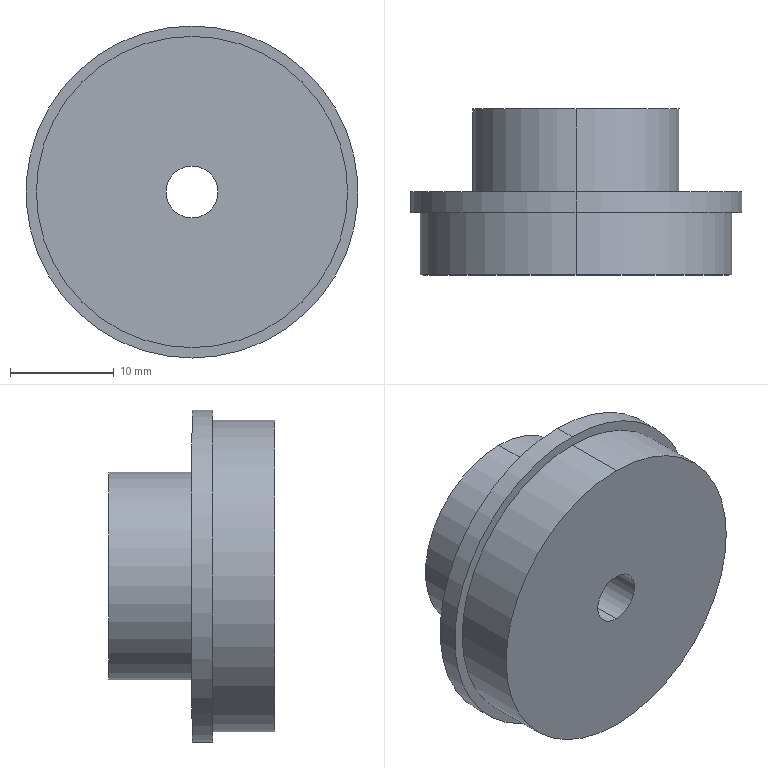Part | STEP file | BCC3 H16_4 | 1 solid | 12 faces | box 32 x 16 x 32 mm | volume 8049 mm3 | cylinder 8 | plane 4 | commonest cylinder face diameters 5 x2 20 x2 30 x2 32 x2
STEP:
#1=CARTESIAN_POINT('',(0.,0.,0.));
#2=DIRECTION('',(0.,0.,1.));
#3=DIRECTION('',(1.,0.,0.));
#4=AXIS2_PLACEMENT_3D('',#1,#2,#3);
#5=CARTESIAN_POINT('',(0.,0.,2.5));
#6=VERTEX_POINT('',#5);
#7=CARTESIAN_POINT('',(0.,16.,2.5));
#8=VERTEX_POINT('',#7);
#9=CARTESIAN_POINT('',(0.,16.,2.5));
#10=DIRECTION('',(0.,1.,0.));
#11=VECTOR('',#10,1.);
#12=LINE('',#9,#11);
#13=CARTESIAN_POINT('',(0.,16.,0.));
#14=DIRECTION('',(0.,1.,0.));
#15=DIRECTION('',(0.,0.,1.));
#16=AXIS2_PLACEMENT_3D('',#13,#14,#15);
#17=CYLINDRICAL_SURFACE('',#16,2.5);
#18=CARTESIAN_POINT('',(6.283,0.));
#19=DIRECTION('',(0.,1.));
#20=VECTOR('',#19,1.);
#21=LINE('',#18,#20);
#22=(GEOMETRIC_REPRESENTATION_CONTEXT(2)PARAMETRIC_REPRESENTATION_CONTEXT()REPRESENTATION_CONTEXT('',''));
#23=DEFINITIONAL_REPRESENTATION('',(#21),#22);
#24=PCURVE('',#17,#23);
#25=CARTESIAN_POINT('',(0.,16.,0.));
#26=DIRECTION('',(0.,1.,0.));
#27=DIRECTION('',(0.,0.,1.));
#28=AXIS2_PLACEMENT_3D('',#25,#26,#27);
#29=CYLINDRICAL_SURFACE('',#28,2.5);
#30=CARTESIAN_POINT('',(0.,0.));
#31=DIRECTION('',(0.,1.));
#32=VECTOR('',#31,1.);
#33=LINE('',#30,#32);
#34=(GEOMETRIC_REPRESENTATION_CONTEXT(2)PARAMETRIC_REPRESENTATION_CONTEXT()REPRESENTATION_CONTEXT('',''));
#35=DEFINITIONAL_REPRESENTATION('',(#33),#34);
#36=PCURVE('',#29,#35);
#37=SURFACE_CURVE('',#12,(#24,#36),.PCURVE_S1.);
#38=EDGE_CURVE('',#6,#8,#37,.T.);
#39=ORIENTED_EDGE('',*,*,#38,.T.);
#40=CARTESIAN_POINT('',(0.,16.,-2.5));
#41=VERTEX_POINT('',#40);
#42=CARTESIAN_POINT('',(0.,16.,0.));
#43=DIRECTION('',(0.,1.,0.));
#44=DIRECTION('',(0.,0.,1.));
#45=AXIS2_PLACEMENT_3D('',#42,#43,#44);
#46=CIRCLE('',#45,2.5);
#47=CARTESIAN_POINT('',(0.,0.));
#48=DIRECTION('',(1.,0.));
#49=VECTOR('',#48,1.);
#50=LINE('',#47,#49);
#51=(GEOMETRIC_REPRESENTATION_CONTEXT(2)PARAMETRIC_REPRESENTATION_CONTEXT()REPRESENTATION_CONTEXT('',''));
#52=DEFINITIONAL_REPRESENTATION('',(#50),#51);
#53=PCURVE('',#17,#52);
#54=CARTESIAN_POINT('',(0.,16.,0.));
#55=DIRECTION('',(0.,1.,0.));
#56=DIRECTION('',(0.,0.,1.));
#57=AXIS2_PLACEMENT_3D('',#54,#55,#56);
#58=PLANE('',#57);
#59=CARTESIAN_POINT('',(0.,0.));
#60=DIRECTION('',(1.,0.));
#61=AXIS2_PLACEMENT_2D('',#59,#60);
#62=CIRCLE('',#61,2.5);
#63=(GEOMETRIC_REPRESENTATION_CONTEXT(2)PARAMETRIC_REPRESENTATION_CONTEXT()REPRESENTATION_CONTEXT('',''));
#64=DEFINITIONAL_REPRESENTATION('',(#62),#63);
#65=PCURVE('',#58,#64);
#66=SURFACE_CURVE('',#46,(#53,#65),.PCURVE_S1.);
#67=EDGE_CURVE('',#41,#8,#66,.T.);
#68=ORIENTED_EDGE('',*,*,#67,.F.);
#69=CARTESIAN_POINT('',(0.,0.,-2.5));
#70=VERTEX_POINT('',#69);
#71=CARTESIAN_POINT('',(0.,16.,-2.5));
#72=DIRECTION('',(0.,1.,0.));
#73=VECTOR('',#72,1.);
#74=LINE('',#71,#73);
#75=CARTESIAN_POINT('',(3.142,0.));
#76=DIRECTION('',(0.,1.));
#77=VECTOR('',#76,1.);
#78=LINE('',#75,#77);
#79=(GEOMETRIC_REPRESENTATION_CONTEXT(2)PARAMETRIC_REPRESENTATION_CONTEXT()REPRESENTATION_CONTEXT('',''));
#80=DEFINITIONAL_REPRESENTATION('',(#78),#79);
#81=PCURVE('',#17,#80);
#82=CARTESIAN_POINT('',(3.142,0.));
#83=DIRECTION('',(0.,1.));
#84=VECTOR('',#83,1.);
#85=LINE('',#82,#84);
#86=(GEOMETRIC_REPRESENTATION_CONTEXT(2)PARAMETRIC_REPRESENTATION_CONTEXT()REPRESENTATION_CONTEXT('',''));
#87=DEFINITIONAL_REPRESENTATION('',(#85),#86);
#88=PCURVE('',#29,#87);
#89=SURFACE_CURVE('',#74,(#81,#88),.PCURVE_S1.);
#90=EDGE_CURVE('',#70,#41,#89,.T.);
#91=ORIENTED_EDGE('',*,*,#90,.F.);
#92=CARTESIAN_POINT('',(0.,0.,0.));
#93=DIRECTION('',(0.,1.,0.));
#94=DIRECTION('',(0.,0.,1.));
#95=AXIS2_PLACEMENT_3D('',#92,#93,#94);
#96=CIRCLE('',#95,2.5);
#97=CARTESIAN_POINT('',(0.,-16.));
#98=DIRECTION('',(1.,0.));
#99=VECTOR('',#98,1.);
#100=LINE('',#97,#99);
#101=(GEOMETRIC_REPRESENTATION_CONTEXT(2)PARAMETRIC_REPRESENTATION_CONTEXT()REPRESENTATION_CONTEXT('',''));
#102=DEFINITIONAL_REPRESENTATION('',(#100),#101);
#103=PCURVE('',#17,#102);
#104=CARTESIAN_POINT('',(0.,0.,0.));
#105=DIRECTION('',(0.,1.,0.));
#106=DIRECTION('',(0.,0.,1.));
#107=AXIS2_PLACEMENT_3D('',#104,#105,#106);
#108=PLANE('',#107);
#109=CARTESIAN_POINT('',(0.,0.));
#110=DIRECTION('',(1.,0.));
#111=AXIS2_PLACEMENT_2D('',#109,#110);
#112=CIRCLE('',#111,2.5);
#113=(GEOMETRIC_REPRESENTATION_CONTEXT(2)PARAMETRIC_REPRESENTATION_CONTEXT()REPRESENTATION_CONTEXT('',''));
#114=DEFINITIONAL_REPRESENTATION('',(#112),#113);
#115=PCURVE('',#108,#114);
#116=SURFACE_CURVE('',#96,(#103,#115),.PCURVE_S1.);
#117=EDGE_CURVE('',#70,#6,#116,.T.);
#118=ORIENTED_EDGE('',*,*,#117,.T.);
#119=EDGE_LOOP('',(#39,#68,#91,#118));
#120=FACE_BOUND('',#119,.F.);
#121=ADVANCED_FACE('',(#120),#17,.F.);
#122=CARTESIAN_POINT('',(0.,16.,10.));
#123=VERTEX_POINT('',#122);
#124=CARTESIAN_POINT('',(0.,16.,-10.));
#125=VERTEX_POINT('',#124);
#126=CARTESIAN_POINT('',(0.,16.,0.));
#127=DIRECTION('',(0.,1.,0.));
#128=DIRECTION('',(0.,0.,1.));
#129=AXIS2_PLACEMENT_3D('',#126,#127,#128);
#130=CIRCLE('',#129,10.);
#131=CARTESIAN_POINT('',(0.,16.,0.));
#132=DIRECTION('',(0.,-1.,0.));
#133=DIRECTION('',(0.,0.,-1.));
#134=AXIS2_PLACEMENT_3D('',#131,#132,#133);
#135=CYLINDRICAL_SURFACE('',#134,10.);
#136=CARTESIAN_POINT('',(3.142,0.));
#137=DIRECTION('',(-1.,0.));
#138=VECTOR('',#137,1.);
#139=LINE('',#136,#138);
#140=(GEOMETRIC_REPRESENTATION_CONTEXT(2)PARAMETRIC_REPRESENTATION_CONTEXT()REPRESENTATION_CONTEXT('',''));
#141=DEFINITIONAL_REPRESENTATION('',(#139),#140);
#142=PCURVE('',#135,#141);
#143=CARTESIAN_POINT('',(0.,0.));
#144=DIRECTION('',(1.,0.));
#145=AXIS2_PLACEMENT_2D('',#143,#144);
#146=CIRCLE('',#145,10.);
#147=(GEOMETRIC_REPRESENTATION_CONTEXT(2)PARAMETRIC_REPRESENTATION_CONTEXT()REPRESENTATION_CONTEXT('',''));
#148=DEFINITIONAL_REPRESENTATION('',(#146),#147);
#149=PCURVE('',#58,#148);
#150=SURFACE_CURVE('',#130,(#142,#149),.PCURVE_S1.);
#151=EDGE_CURVE('',#123,#125,#150,.T.);
#152=ORIENTED_EDGE('',*,*,#151,.F.);
#153=CARTESIAN_POINT('',(0.,8.,10.));
#154=VERTEX_POINT('',#153);
#155=CARTESIAN_POINT('',(0.,16.,10.));
#156=DIRECTION('',(0.,-1.,0.));
#157=VECTOR('',#156,1.);
#158=LINE('',#155,#157);
#159=CARTESIAN_POINT('',(3.142,0.));
#160=DIRECTION('',(0.,1.));
#161=VECTOR('',#160,1.);
#162=LINE('',#159,#161);
#163=(GEOMETRIC_REPRESENTATION_CONTEXT(2)PARAMETRIC_REPRESENTATION_CONTEXT()REPRESENTATION_CONTEXT('',''));
#164=DEFINITIONAL_REPRESENTATION('',(#162),#163);
#165=PCURVE('',#135,#164);
#166=CARTESIAN_POINT('',(0.,16.,0.));
#167=DIRECTION('',(0.,-1.,0.));
#168=DIRECTION('',(0.,0.,-1.));
#169=AXIS2_PLACEMENT_3D('',#166,#167,#168);
#170=CYLINDRICAL_SURFACE('',#169,10.);
#171=CARTESIAN_POINT('',(3.142,0.));
#172=DIRECTION('',(0.,1.));
#173=VECTOR('',#172,1.);
#174=LINE('',#171,#173);
#175=(GEOMETRIC_REPRESENTATION_CONTEXT(2)PARAMETRIC_REPRESENTATION_CONTEXT()REPRESENTATION_CONTEXT('',''));
#176=DEFINITIONAL_REPRESENTATION('',(#174),#175);
#177=PCURVE('',#170,#176);
#178=SURFACE_CURVE('',#158,(#165,#177),.PCURVE_S1.);
#179=EDGE_CURVE('',#123,#154,#178,.T.);
#180=ORIENTED_EDGE('',*,*,#179,.T.);
#181=CARTESIAN_POINT('',(0.,8.,-10.));
#182=VERTEX_POINT('',#181);
#183=CARTESIAN_POINT('',(0.,8.,0.));
#184=DIRECTION('',(0.,1.,0.));
#185=DIRECTION('',(0.,0.,1.));
#186=AXIS2_PLACEMENT_3D('',#183,#184,#185);
#187=CIRCLE('',#186,10.);
#188=CARTESIAN_POINT('',(3.142,8.));
#189=DIRECTION('',(-1.,0.));
#190=VECTOR('',#189,1.);
#191=LINE('',#188,#190);
#192=(GEOMETRIC_REPRESENTATION_CONTEXT(2)PARAMETRIC_REPRESENTATION_CONTEXT()REPRESENTATION_CONTEXT('',''));
#193=DEFINITIONAL_REPRESENTATION('',(#191),#192);
#194=PCURVE('',#135,#193);
#195=CARTESIAN_POINT('',(0.,8.,0.));
#196=DIRECTION('',(0.,1.,0.));
#197=DIRECTION('',(0.,0.,1.));
#198=AXIS2_PLACEMENT_3D('',#195,#196,#197);
#199=PLANE('',#198);
#200=CARTESIAN_POINT('',(0.,0.));
#201=DIRECTION('',(1.,0.));
#202=AXIS2_PLACEMENT_2D('',#200,#201);
#203=CIRCLE('',#202,10.);
#204=(GEOMETRIC_REPRESENTATION_CONTEXT(2)PARAMETRIC_REPRESENTATION_CONTEXT()REPRESENTATION_CONTEXT('',''));
#205=DEFINITIONAL_REPRESENTATION('',(#203),#204);
#206=PCURVE('',#199,#205);
#207=SURFACE_CURVE('',#187,(#194,#206),.PCURVE_S1.);
#208=EDGE_CURVE('',#154,#182,#207,.T.);
#209=ORIENTED_EDGE('',*,*,#208,.T.);
#210=CARTESIAN_POINT('',(0.,16.,-10.));
#211=DIRECTION('',(0.,-1.,0.));
#212=VECTOR('',#211,1.);
#213=LINE('',#210,#212);
#214=CARTESIAN_POINT('',(0.,0.));
#215=DIRECTION('',(0.,1.));
#216=VECTOR('',#215,1.);
#217=LINE('',#214,#216);
#218=(GEOMETRIC_REPRESENTATION_CONTEXT(2)PARAMETRIC_REPRESENTATION_CONTEXT()REPRESENTATION_CONTEXT('',''));
#219=DEFINITIONAL_REPRESENTATION('',(#217),#218);
#220=PCURVE('',#135,#219);
#221=CARTESIAN_POINT('',(6.283,0.));
#222=DIRECTION('',(0.,1.));
#223=VECTOR('',#222,1.);
#224=LINE('',#221,#223);
#225=(GEOMETRIC_REPRESENTATION_CONTEXT(2)PARAMETRIC_REPRESENTATION_CONTEXT()REPRESENTATION_CONTEXT('',''));
#226=DEFINITIONAL_REPRESENTATION('',(#224),#225);
#227=PCURVE('',#170,#226);
#228=SURFACE_CURVE('',#213,(#220,#227),.PCURVE_S1.);
#229=EDGE_CURVE('',#125,#182,#228,.T.);
#230=ORIENTED_EDGE('',*,*,#229,.F.);
#231=EDGE_LOOP('',(#152,#180,#209,#230));
#232=FACE_BOUND('',#231,.T.);
#233=ADVANCED_FACE('',(#232),#135,.T.);
#234=CARTESIAN_POINT('',(0.,8.,16.));
#235=VERTEX_POINT('',#234);
#236=CARTESIAN_POINT('',(0.,8.,-16.));
#237=VERTEX_POINT('',#236);
#238=CARTESIAN_POINT('',(0.,8.,0.));
#239=DIRECTION('',(0.,1.,0.));
#240=DIRECTION('',(0.,0.,1.));
#241=AXIS2_PLACEMENT_3D('',#238,#239,#240);
#242=CIRCLE('',#241,16.);
#243=CARTESIAN_POINT('',(0.,8.,0.));
#244=DIRECTION('',(0.,-1.,0.));
#245=DIRECTION('',(0.,0.,-1.));
#246=AXIS2_PLACEMENT_3D('',#243,#244,#245);
#247=CYLINDRICAL_SURFACE('',#246,16.);
#248=CARTESIAN_POINT('',(3.142,0.));
#249=DIRECTION('',(-1.,0.));
#250=VECTOR('',#249,1.);
#251=LINE('',#248,#250);
#252=(GEOMETRIC_REPRESENTATION_CONTEXT(2)PARAMETRIC_REPRESENTATION_CONTEXT()REPRESENTATION_CONTEXT('',''));
#253=DEFINITIONAL_REPRESENTATION('',(#251),#252);
#254=PCURVE('',#247,#253);
#255=CARTESIAN_POINT('',(0.,0.));
#256=DIRECTION('',(1.,0.));
#257=AXIS2_PLACEMENT_2D('',#255,#256);
#258=CIRCLE('',#257,16.);
#259=(GEOMETRIC_REPRESENTATION_CONTEXT(2)PARAMETRIC_REPRESENTATION_CONTEXT()REPRESENTATION_CONTEXT('',''));
#260=DEFINITIONAL_REPRESENTATION('',(#258),#259);
#261=PCURVE('',#199,#260);
#262=SURFACE_CURVE('',#242,(#254,#261),.PCURVE_S1.);
#263=EDGE_CURVE('',#235,#237,#262,.T.);
#264=ORIENTED_EDGE('',*,*,#263,.F.);
#265=CARTESIAN_POINT('',(0.,6.,16.));
#266=VERTEX_POINT('',#265);
#267=CARTESIAN_POINT('',(0.,8.,16.));
#268=DIRECTION('',(0.,-1.,0.));
#269=VECTOR('',#268,1.);
#270=LINE('',#267,#269);
#271=CARTESIAN_POINT('',(3.142,0.));
#272=DIRECTION('',(0.,1.));
#273=VECTOR('',#272,1.);
#274=LINE('',#271,#273);
#275=(GEOMETRIC_REPRESENTATION_CONTEXT(2)PARAMETRIC_REPRESENTATION_CONTEXT()REPRESENTATION_CONTEXT('',''));
#276=DEFINITIONAL_REPRESENTATION('',(#274),#275);
#277=PCURVE('',#247,#276);
#278=CARTESIAN_POINT('',(0.,8.,0.));
#279=DIRECTION('',(0.,-1.,0.));
#280=DIRECTION('',(0.,0.,-1.));
#281=AXIS2_PLACEMENT_3D('',#278,#279,#280);
#282=CYLINDRICAL_SURFACE('',#281,16.);
#283=CARTESIAN_POINT('',(3.142,0.));
#284=DIRECTION('',(0.,1.));
#285=VECTOR('',#284,1.);
#286=LINE('',#283,#285);
#287=(GEOMETRIC_REPRESENTATION_CONTEXT(2)PARAMETRIC_REPRESENTATION_CONTEXT()REPRESENTATION_CONTEXT('',''));
#288=DEFINITIONAL_REPRESENTATION('',(#286),#287);
#289=PCURVE('',#282,#288);
#290=SURFACE_CURVE('',#270,(#277,#289),.PCURVE_S1.);
#291=EDGE_CURVE('',#235,#266,#290,.T.);
#292=ORIENTED_EDGE('',*,*,#291,.T.);
#293=CARTESIAN_POINT('',(0.,6.,-16.));
#294=VERTEX_POINT('',#293);
#295=CARTESIAN_POINT('',(0.,6.,0.));
#296=DIRECTION('',(0.,1.,0.));
#297=DIRECTION('',(0.,0.,1.));
#298=AXIS2_PLACEMENT_3D('',#295,#296,#297);
#299=CIRCLE('',#298,16.);
#300=CARTESIAN_POINT('',(3.142,2.));
#301=DIRECTION('',(-1.,0.));
#302=VECTOR('',#301,1.);
#303=LINE('',#300,#302);
#304=(GEOMETRIC_REPRESENTATION_CONTEXT(2)PARAMETRIC_REPRESENTATION_CONTEXT()REPRESENTATION_CONTEXT('',''));
#305=DEFINITIONAL_REPRESENTATION('',(#303),#304);
#306=PCURVE('',#247,#305);
#307=CARTESIAN_POINT('',(0.,6.,0.));
#308=DIRECTION('',(0.,1.,0.));
#309=DIRECTION('',(0.,0.,1.));
#310=AXIS2_PLACEMENT_3D('',#307,#308,#309);
#311=PLANE('',#310);
#312=CARTESIAN_POINT('',(0.,0.));
#313=DIRECTION('',(1.,0.));
#314=AXIS2_PLACEMENT_2D('',#312,#313);
#315=CIRCLE('',#314,16.);
#316=(GEOMETRIC_REPRESENTATION_CONTEXT(2)PARAMETRIC_REPRESENTATION_CONTEXT()REPRESENTATION_CONTEXT('',''));
#317=DEFINITIONAL_REPRESENTATION('',(#315),#316);
#318=PCURVE('',#311,#317);
#319=SURFACE_CURVE('',#299,(#306,#318),.PCURVE_S1.);
#320=EDGE_CURVE('',#266,#294,#319,.T.);
#321=ORIENTED_EDGE('',*,*,#320,.T.);
#322=CARTESIAN_POINT('',(0.,8.,-16.));
#323=DIRECTION('',(0.,-1.,0.));
#324=VECTOR('',#323,1.);
#325=LINE('',#322,#324);
#326=CARTESIAN_POINT('',(0.,0.));
#327=DIRECTION('',(0.,1.));
#328=VECTOR('',#327,1.);
#329=LINE('',#326,#328);
#330=(GEOMETRIC_REPRESENTATION_CONTEXT(2)PARAMETRIC_REPRESENTATION_CONTEXT()REPRESENTATION_CONTEXT('',''));
#331=DEFINITIONAL_REPRESENTATION('',(#329),#330);
#332=PCURVE('',#247,#331);
#333=CARTESIAN_POINT('',(6.283,0.));
#334=DIRECTION('',(0.,1.));
#335=VECTOR('',#334,1.);
#336=LINE('',#333,#335);
#337=(GEOMETRIC_REPRESENTATION_CONTEXT(2)PARAMETRIC_REPRESENTATION_CONTEXT()REPRESENTATION_CONTEXT('',''));
#338=DEFINITIONAL_REPRESENTATION('',(#336),#337);
#339=PCURVE('',#282,#338);
#340=SURFACE_CURVE('',#325,(#332,#339),.PCURVE_S1.);
#341=EDGE_CURVE('',#237,#294,#340,.T.);
#342=ORIENTED_EDGE('',*,*,#341,.F.);
#343=EDGE_LOOP('',(#264,#292,#321,#342));
#344=FACE_BOUND('',#343,.T.);
#345=ADVANCED_FACE('',(#344),#247,.T.);
#346=CARTESIAN_POINT('',(0.,6.,15.));
#347=VERTEX_POINT('',#346);
#348=CARTESIAN_POINT('',(0.,6.,-15.));
#349=VERTEX_POINT('',#348);
#350=CARTESIAN_POINT('',(0.,6.,0.));
#351=DIRECTION('',(0.,1.,0.));
#352=DIRECTION('',(0.,0.,1.));
#353=AXIS2_PLACEMENT_3D('',#350,#351,#352);
#354=CIRCLE('',#353,15.);
#355=CARTESIAN_POINT('',(0.,6.,0.));
#356=DIRECTION('',(0.,-1.,0.));
#357=DIRECTION('',(0.,0.,-1.));
#358=AXIS2_PLACEMENT_3D('',#355,#356,#357);
#359=CYLINDRICAL_SURFACE('',#358,15.);
#360=CARTESIAN_POINT('',(3.142,0.));
#361=DIRECTION('',(-1.,0.));
#362=VECTOR('',#361,1.);
#363=LINE('',#360,#362);
#364=(GEOMETRIC_REPRESENTATION_CONTEXT(2)PARAMETRIC_REPRESENTATION_CONTEXT()REPRESENTATION_CONTEXT('',''));
#365=DEFINITIONAL_REPRESENTATION('',(#363),#364);
#366=PCURVE('',#359,#365);
#367=CARTESIAN_POINT('',(0.,0.));
#368=DIRECTION('',(1.,0.));
#369=AXIS2_PLACEMENT_2D('',#367,#368);
#370=CIRCLE('',#369,15.);
#371=(GEOMETRIC_REPRESENTATION_CONTEXT(2)PARAMETRIC_REPRESENTATION_CONTEXT()REPRESENTATION_CONTEXT('',''));
#372=DEFINITIONAL_REPRESENTATION('',(#370),#371);
#373=PCURVE('',#311,#372);
#374=SURFACE_CURVE('',#354,(#366,#373),.PCURVE_S1.);
#375=EDGE_CURVE('',#347,#349,#374,.T.);
#376=ORIENTED_EDGE('',*,*,#375,.F.);
#377=CARTESIAN_POINT('',(0.,0.,15.));
#378=VERTEX_POINT('',#377);
#379=CARTESIAN_POINT('',(0.,6.,15.));
#380=DIRECTION('',(0.,-1.,0.));
#381=VECTOR('',#380,1.);
#382=LINE('',#379,#381);
#383=CARTESIAN_POINT('',(3.142,0.));
#384=DIRECTION('',(0.,1.));
#385=VECTOR('',#384,1.);
#386=LINE('',#383,#385);
#387=(GEOMETRIC_REPRESENTATION_CONTEXT(2)PARAMETRIC_REPRESENTATION_CONTEXT()REPRESENTATION_CONTEXT('',''));
#388=DEFINITIONAL_REPRESENTATION('',(#386),#387);
#389=PCURVE('',#359,#388);
#390=CARTESIAN_POINT('',(0.,6.,0.));
#391=DIRECTION('',(0.,-1.,0.));
#392=DIRECTION('',(0.,0.,-1.));
#393=AXIS2_PLACEMENT_3D('',#390,#391,#392);
#394=CYLINDRICAL_SURFACE('',#393,15.);
#395=CARTESIAN_POINT('',(3.142,0.));
#396=DIRECTION('',(0.,1.));
#397=VECTOR('',#396,1.);
#398=LINE('',#395,#397);
#399=(GEOMETRIC_REPRESENTATION_CONTEXT(2)PARAMETRIC_REPRESENTATION_CONTEXT()REPRESENTATION_CONTEXT('',''));
#400=DEFINITIONAL_REPRESENTATION('',(#398),#399);
#401=PCURVE('',#394,#400);
#402=SURFACE_CURVE('',#382,(#389,#401),.PCURVE_S1.);
#403=EDGE_CURVE('',#347,#378,#402,.T.);
#404=ORIENTED_EDGE('',*,*,#403,.T.);
#405=CARTESIAN_POINT('',(0.,0.,-15.));
#406=VERTEX_POINT('',#405);
#407=CARTESIAN_POINT('',(0.,0.,0.));
#408=DIRECTION('',(0.,1.,0.));
#409=DIRECTION('',(0.,0.,1.));
#410=AXIS2_PLACEMENT_3D('',#407,#408,#409);
#411=CIRCLE('',#410,15.);
#412=CARTESIAN_POINT('',(3.142,6.));
#413=DIRECTION('',(-1.,0.));
#414=VECTOR('',#413,1.);
#415=LINE('',#412,#414);
#416=(GEOMETRIC_REPRESENTATION_CONTEXT(2)PARAMETRIC_REPRESENTATION_CONTEXT()REPRESENTATION_CONTEXT('',''));
#417=DEFINITIONAL_REPRESENTATION('',(#415),#416);
#418=PCURVE('',#359,#417);
#419=CARTESIAN_POINT('',(0.,0.));
#420=DIRECTION('',(1.,0.));
#421=AXIS2_PLACEMENT_2D('',#419,#420);
#422=CIRCLE('',#421,15.);
#423=(GEOMETRIC_REPRESENTATION_CONTEXT(2)PARAMETRIC_REPRESENTATION_CONTEXT()REPRESENTATION_CONTEXT('',''));
#424=DEFINITIONAL_REPRESENTATION('',(#422),#423);
#425=PCURVE('',#108,#424);
#426=SURFACE_CURVE('',#411,(#418,#425),.PCURVE_S1.);
#427=EDGE_CURVE('',#378,#406,#426,.T.);
#428=ORIENTED_EDGE('',*,*,#427,.T.);
#429=CARTESIAN_POINT('',(0.,6.,-15.));
#430=DIRECTION('',(0.,-1.,0.));
#431=VECTOR('',#430,1.);
#432=LINE('',#429,#431);
#433=CARTESIAN_POINT('',(0.,0.));
#434=DIRECTION('',(0.,1.));
#435=VECTOR('',#434,1.);
#436=LINE('',#433,#435);
#437=(GEOMETRIC_REPRESENTATION_CONTEXT(2)PARAMETRIC_REPRESENTATION_CONTEXT()REPRESENTATION_CONTEXT('',''));
#438=DEFINITIONAL_REPRESENTATION('',(#436),#437);
#439=PCURVE('',#359,#438);
#440=CARTESIAN_POINT('',(6.283,0.));
#441=DIRECTION('',(0.,1.));
#442=VECTOR('',#441,1.);
#443=LINE('',#440,#442);
#444=(GEOMETRIC_REPRESENTATION_CONTEXT(2)PARAMETRIC_REPRESENTATION_CONTEXT()REPRESENTATION_CONTEXT('',''));
#445=DEFINITIONAL_REPRESENTATION('',(#443),#444);
#446=PCURVE('',#394,#445);
#447=SURFACE_CURVE('',#432,(#439,#446),.PCURVE_S1.);
#448=EDGE_CURVE('',#349,#406,#447,.T.);
#449=ORIENTED_EDGE('',*,*,#448,.F.);
#450=EDGE_LOOP('',(#376,#404,#428,#449));
#451=FACE_BOUND('',#450,.T.);
#452=ADVANCED_FACE('',(#451),#359,.T.);
#453=CARTESIAN_POINT('',(0.,8.,0.));
#454=DIRECTION('',(0.,1.,0.));
#455=DIRECTION('',(0.,0.,1.));
#456=AXIS2_PLACEMENT_3D('',#453,#454,#455);
#457=CIRCLE('',#456,16.);
#458=CARTESIAN_POINT('',(0.,0.));
#459=DIRECTION('',(1.,0.));
#460=AXIS2_PLACEMENT_2D('',#458,#459);
#461=CIRCLE('',#460,16.);
#462=(GEOMETRIC_REPRESENTATION_CONTEXT(2)PARAMETRIC_REPRESENTATION_CONTEXT()REPRESENTATION_CONTEXT('',''));
#463=DEFINITIONAL_REPRESENTATION('',(#461),#462);
#464=PCURVE('',#199,#463);
#465=CARTESIAN_POINT('',(9.425,0.));
#466=DIRECTION('',(-1.,0.));
#467=VECTOR('',#466,1.);
#468=LINE('',#465,#467);
#469=(GEOMETRIC_REPRESENTATION_CONTEXT(2)PARAMETRIC_REPRESENTATION_CONTEXT()REPRESENTATION_CONTEXT('',''));
#470=DEFINITIONAL_REPRESENTATION('',(#468),#469);
#471=PCURVE('',#282,#470);
#472=SURFACE_CURVE('',#457,(#464,#471),.PCURVE_S1.);
#473=EDGE_CURVE('',#237,#235,#472,.T.);
#474=ORIENTED_EDGE('',*,*,#473,.T.);
#475=ORIENTED_EDGE('',*,*,#263,.T.);
#476=EDGE_LOOP('',(#474,#475));
#477=FACE_BOUND('',#476,.T.);
#478=CARTESIAN_POINT('',(0.,8.,0.));
#479=DIRECTION('',(0.,1.,0.));
#480=DIRECTION('',(0.,0.,1.));
#481=AXIS2_PLACEMENT_3D('',#478,#479,#480);
#482=CIRCLE('',#481,10.);
#483=CARTESIAN_POINT('',(0.,0.));
#484=DIRECTION('',(1.,0.));
#485=AXIS2_PLACEMENT_2D('',#483,#484);
#486=CIRCLE('',#485,10.);
#487=(GEOMETRIC_REPRESENTATION_CONTEXT(2)PARAMETRIC_REPRESENTATION_CONTEXT()REPRESENTATION_CONTEXT('',''));
#488=DEFINITIONAL_REPRESENTATION('',(#486),#487);
#489=PCURVE('',#199,#488);
#490=CARTESIAN_POINT('',(9.425,8.));
#491=DIRECTION('',(-1.,0.));
#492=VECTOR('',#491,1.);
#493=LINE('',#490,#492);
#494=(GEOMETRIC_REPRESENTATION_CONTEXT(2)PARAMETRIC_REPRESENTATION_CONTEXT()REPRESENTATION_CONTEXT('',''));
#495=DEFINITIONAL_REPRESENTATION('',(#493),#494);
#496=PCURVE('',#170,#495);
#497=SURFACE_CURVE('',#482,(#489,#496),.PCURVE_S1.);
#498=EDGE_CURVE('',#182,#154,#497,.T.);
#499=ORIENTED_EDGE('',*,*,#498,.F.);
#500=ORIENTED_EDGE('',*,*,#208,.F.);
#501=EDGE_LOOP('',(#499,#500));
#502=FACE_BOUND('',#501,.T.);
#503=ADVANCED_FACE('',(#477,#502),#199,.T.);
#504=ORIENTED_EDGE('',*,*,#403,.F.);
#505=CARTESIAN_POINT('',(0.,6.,0.));
#506=DIRECTION('',(0.,1.,0.));
#507=DIRECTION('',(0.,0.,1.));
#508=AXIS2_PLACEMENT_3D('',#505,#506,#507);
#509=CIRCLE('',#508,15.);
#510=CARTESIAN_POINT('',(9.425,0.));
#511=DIRECTION('',(-1.,0.));
#512=VECTOR('',#511,1.);
#513=LINE('',#510,#512);
#514=(GEOMETRIC_REPRESENTATION_CONTEXT(2)PARAMETRIC_REPRESENTATION_CONTEXT()REPRESENTATION_CONTEXT('',''));
#515=DEFINITIONAL_REPRESENTATION('',(#513),#514);
#516=PCURVE('',#394,#515);
#517=CARTESIAN_POINT('',(0.,0.));
#518=DIRECTION('',(1.,0.));
#519=AXIS2_PLACEMENT_2D('',#517,#518);
#520=CIRCLE('',#519,15.);
#521=(GEOMETRIC_REPRESENTATION_CONTEXT(2)PARAMETRIC_REPRESENTATION_CONTEXT()REPRESENTATION_CONTEXT('',''));
#522=DEFINITIONAL_REPRESENTATION('',(#520),#521);
#523=PCURVE('',#311,#522);
#524=SURFACE_CURVE('',#509,(#516,#523),.PCURVE_S1.);
#525=EDGE_CURVE('',#349,#347,#524,.T.);
#526=ORIENTED_EDGE('',*,*,#525,.F.);
#527=ORIENTED_EDGE('',*,*,#448,.T.);
#528=CARTESIAN_POINT('',(0.,0.,0.));
#529=DIRECTION('',(0.,1.,0.));
#530=DIRECTION('',(0.,0.,1.));
#531=AXIS2_PLACEMENT_3D('',#528,#529,#530);
#532=CIRCLE('',#531,15.);
#533=CARTESIAN_POINT('',(9.425,6.));
#534=DIRECTION('',(-1.,0.));
#535=VECTOR('',#534,1.);
#536=LINE('',#533,#535);
#537=(GEOMETRIC_REPRESENTATION_CONTEXT(2)PARAMETRIC_REPRESENTATION_CONTEXT()REPRESENTATION_CONTEXT('',''));
#538=DEFINITIONAL_REPRESENTATION('',(#536),#537);
#539=PCURVE('',#394,#538);
#540=CARTESIAN_POINT('',(0.,0.));
#541=DIRECTION('',(1.,0.));
#542=AXIS2_PLACEMENT_2D('',#540,#541);
#543=CIRCLE('',#542,15.);
#544=(GEOMETRIC_REPRESENTATION_CONTEXT(2)PARAMETRIC_REPRESENTATION_CONTEXT()REPRESENTATION_CONTEXT('',''));
#545=DEFINITIONAL_REPRESENTATION('',(#543),#544);
#546=PCURVE('',#108,#545);
#547=SURFACE_CURVE('',#532,(#539,#546),.PCURVE_S1.);
#548=EDGE_CURVE('',#406,#378,#547,.T.);
#549=ORIENTED_EDGE('',*,*,#548,.T.);
#550=EDGE_LOOP('',(#504,#526,#527,#549));
#551=FACE_BOUND('',#550,.T.);
#552=ADVANCED_FACE('',(#551),#394,.T.);
#553=CARTESIAN_POINT('',(0.,0.,0.));
#554=DIRECTION('',(0.,1.,0.));
#555=DIRECTION('',(0.,0.,1.));
#556=AXIS2_PLACEMENT_3D('',#553,#554,#555);
#557=CIRCLE('',#556,2.5);
#558=CARTESIAN_POINT('',(0.,0.));
#559=DIRECTION('',(1.,0.));
#560=AXIS2_PLACEMENT_2D('',#558,#559);
#561=CIRCLE('',#560,2.5);
#562=(GEOMETRIC_REPRESENTATION_CONTEXT(2)PARAMETRIC_REPRESENTATION_CONTEXT()REPRESENTATION_CONTEXT('',''));
#563=DEFINITIONAL_REPRESENTATION('',(#561),#562);
#564=PCURVE('',#108,#563);
#565=CARTESIAN_POINT('',(0.,-16.));
#566=DIRECTION('',(1.,0.));
#567=VECTOR('',#566,1.);
#568=LINE('',#565,#567);
#569=(GEOMETRIC_REPRESENTATION_CONTEXT(2)PARAMETRIC_REPRESENTATION_CONTEXT()REPRESENTATION_CONTEXT('',''));
#570=DEFINITIONAL_REPRESENTATION('',(#568),#569);
#571=PCURVE('',#29,#570);
#572=SURFACE_CURVE('',#557,(#564,#571),.PCURVE_S1.);
#573=EDGE_CURVE('',#6,#70,#572,.T.);
#574=ORIENTED_EDGE('',*,*,#573,.T.);
#575=ORIENTED_EDGE('',*,*,#117,.T.);
#576=EDGE_LOOP('',(#574,#575));
#577=FACE_BOUND('',#576,.T.);
#578=ORIENTED_EDGE('',*,*,#548,.F.);
#579=ORIENTED_EDGE('',*,*,#427,.F.);
#580=EDGE_LOOP('',(#578,#579));
#581=FACE_BOUND('',#580,.T.);
#582=ADVANCED_FACE('',(#577,#581),#108,.F.);
#583=CARTESIAN_POINT('',(0.,6.,0.));
#584=DIRECTION('',(0.,1.,0.));
#585=DIRECTION('',(0.,0.,1.));
#586=AXIS2_PLACEMENT_3D('',#583,#584,#585);
#587=CIRCLE('',#586,16.);
#588=CARTESIAN_POINT('',(0.,0.));
#589=DIRECTION('',(1.,0.));
#590=AXIS2_PLACEMENT_2D('',#588,#589);
#591=CIRCLE('',#590,16.);
#592=(GEOMETRIC_REPRESENTATION_CONTEXT(2)PARAMETRIC_REPRESENTATION_CONTEXT()REPRESENTATION_CONTEXT('',''));
#593=DEFINITIONAL_REPRESENTATION('',(#591),#592);
#594=PCURVE('',#311,#593);
#595=CARTESIAN_POINT('',(9.425,2.));
#596=DIRECTION('',(-1.,0.));
#597=VECTOR('',#596,1.);
#598=LINE('',#595,#597);
#599=(GEOMETRIC_REPRESENTATION_CONTEXT(2)PARAMETRIC_REPRESENTATION_CONTEXT()REPRESENTATION_CONTEXT('',''));
#600=DEFINITIONAL_REPRESENTATION('',(#598),#599);
#601=PCURVE('',#282,#600);
#602=SURFACE_CURVE('',#587,(#594,#601),.PCURVE_S1.);
#603=EDGE_CURVE('',#294,#266,#602,.T.);
#604=ORIENTED_EDGE('',*,*,#603,.F.);
#605=ORIENTED_EDGE('',*,*,#320,.F.);
#606=EDGE_LOOP('',(#604,#605));
#607=FACE_BOUND('',#606,.T.);
#608=ORIENTED_EDGE('',*,*,#525,.T.);
#609=ORIENTED_EDGE('',*,*,#375,.T.);
#610=EDGE_LOOP('',(#608,#609));
#611=FACE_BOUND('',#610,.T.);
#612=ADVANCED_FACE('',(#607,#611),#311,.F.);
#613=ORIENTED_EDGE('',*,*,#291,.F.);
#614=ORIENTED_EDGE('',*,*,#473,.F.);
#615=ORIENTED_EDGE('',*,*,#341,.T.);
#616=ORIENTED_EDGE('',*,*,#603,.T.);
#617=EDGE_LOOP('',(#613,#614,#615,#616));
#618=FACE_BOUND('',#617,.T.);
#619=ADVANCED_FACE('',(#618),#282,.T.);
#620=ORIENTED_EDGE('',*,*,#179,.F.);
#621=CARTESIAN_POINT('',(0.,16.,0.));
#622=DIRECTION('',(0.,1.,0.));
#623=DIRECTION('',(0.,0.,1.));
#624=AXIS2_PLACEMENT_3D('',#621,#622,#623);
#625=CIRCLE('',#624,10.);
#626=CARTESIAN_POINT('',(9.425,0.));
#627=DIRECTION('',(-1.,0.));
#628=VECTOR('',#627,1.);
#629=LINE('',#626,#628);
#630=(GEOMETRIC_REPRESENTATION_CONTEXT(2)PARAMETRIC_REPRESENTATION_CONTEXT()REPRESENTATION_CONTEXT('',''));
#631=DEFINITIONAL_REPRESENTATION('',(#629),#630);
#632=PCURVE('',#170,#631);
#633=CARTESIAN_POINT('',(0.,0.));
#634=DIRECTION('',(1.,0.));
#635=AXIS2_PLACEMENT_2D('',#633,#634);
#636=CIRCLE('',#635,10.);
#637=(GEOMETRIC_REPRESENTATION_CONTEXT(2)PARAMETRIC_REPRESENTATION_CONTEXT()REPRESENTATION_CONTEXT('',''));
#638=DEFINITIONAL_REPRESENTATION('',(#636),#637);
#639=PCURVE('',#58,#638);
#640=SURFACE_CURVE('',#625,(#632,#639),.PCURVE_S1.);
#641=EDGE_CURVE('',#125,#123,#640,.T.);
#642=ORIENTED_EDGE('',*,*,#641,.F.);
#643=ORIENTED_EDGE('',*,*,#229,.T.);
#644=ORIENTED_EDGE('',*,*,#498,.T.);
#645=EDGE_LOOP('',(#620,#642,#643,#644));
#646=FACE_BOUND('',#645,.T.);
#647=ADVANCED_FACE('',(#646),#170,.T.);
#648=CARTESIAN_POINT('',(0.,16.,0.));
#649=DIRECTION('',(0.,1.,0.));
#650=DIRECTION('',(0.,0.,1.));
#651=AXIS2_PLACEMENT_3D('',#648,#649,#650);
#652=CIRCLE('',#651,2.5);
#653=CARTESIAN_POINT('',(0.,0.));
#654=DIRECTION('',(1.,0.));
#655=AXIS2_PLACEMENT_2D('',#653,#654);
#656=CIRCLE('',#655,2.5);
#657=(GEOMETRIC_REPRESENTATION_CONTEXT(2)PARAMETRIC_REPRESENTATION_CONTEXT()REPRESENTATION_CONTEXT('',''));
#658=DEFINITIONAL_REPRESENTATION('',(#656),#657);
#659=PCURVE('',#58,#658);
#660=CARTESIAN_POINT('',(0.,0.));
#661=DIRECTION('',(1.,0.));
#662=VECTOR('',#661,1.);
#663=LINE('',#660,#662);
#664=(GEOMETRIC_REPRESENTATION_CONTEXT(2)PARAMETRIC_REPRESENTATION_CONTEXT()REPRESENTATION_CONTEXT('',''));
#665=DEFINITIONAL_REPRESENTATION('',(#663),#664);
#666=PCURVE('',#29,#665);
#667=SURFACE_CURVE('',#652,(#659,#666),.PCURVE_S1.);
#668=EDGE_CURVE('',#8,#41,#667,.T.);
#669=ORIENTED_EDGE('',*,*,#668,.F.);
#670=ORIENTED_EDGE('',*,*,#67,.F.);
#671=EDGE_LOOP('',(#669,#670));
#672=FACE_BOUND('',#671,.T.);
#673=ORIENTED_EDGE('',*,*,#641,.T.);
#674=ORIENTED_EDGE('',*,*,#151,.T.);
#675=EDGE_LOOP('',(#673,#674));
#676=FACE_BOUND('',#675,.T.);
#677=ADVANCED_FACE('',(#672,#676),#58,.T.);
#678=ORIENTED_EDGE('',*,*,#668,.F.);
#679=ORIENTED_EDGE('',*,*,#38,.F.);
#680=ORIENTED_EDGE('',*,*,#573,.T.);
#681=ORIENTED_EDGE('',*,*,#90,.T.);
#682=EDGE_LOOP('',(#678,#679,#680,#681));
#683=FACE_BOUND('',#682,.F.);
#684=ADVANCED_FACE('',(#683),#29,.F.);
#685=CLOSED_SHELL('',(#121,#233,#345,#452,#503,#552,#582,#612,#619,#647,#677,#684));
#686=MANIFOLD_SOLID_BREP('',#685);
#687=(LENGTH_UNIT()NAMED_UNIT(*)SI_UNIT(.MILLI.,.METRE.));
#688=UNCERTAINTY_MEASURE_WITH_UNIT(LENGTH_MEASURE(0.0000001),#687,'','');
#689=(NAMED_UNIT(*)PLANE_ANGLE_UNIT()SI_UNIT($,.RADIAN.));
#690=(NAMED_UNIT(*)SI_UNIT($,.STERADIAN.)SOLID_ANGLE_UNIT());
#691=(GEOMETRIC_REPRESENTATION_CONTEXT(3)GLOBAL_UNCERTAINTY_ASSIGNED_CONTEXT((#688))GLOBAL_UNIT_ASSIGNED_CONTEXT((#687,#689,#690))REPRESENTATION_CONTEXT('',''));
#692=ADVANCED_BREP_SHAPE_REPRESENTATION('',(#4,#686),#691);